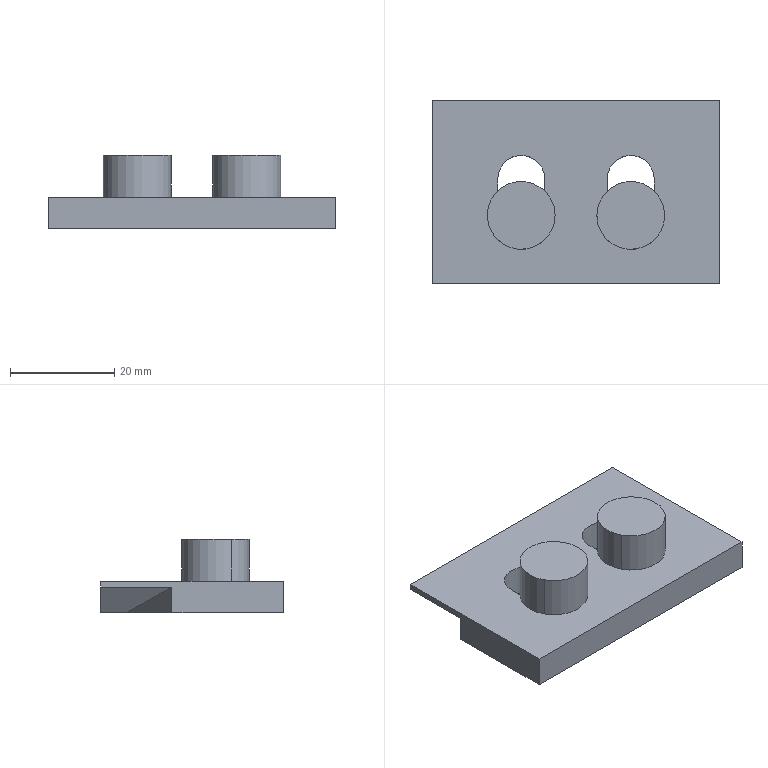Part | CATIA | 3 solids | 26 faces | box 55 x 35 x 14 mm | volume 11367 mm3 | plane 18 | cylinder 8 | commonest cylinder face diameters 9 x4 13 x4
STEP:
#1=CARTESIAN_POINT('',(-27.5,-30.,38.));
#2=VERTEX_POINT('',#1);
#3=CARTESIAN_POINT('',(-27.5,-30.,44.));
#4=VERTEX_POINT('',#3);
#5=CARTESIAN_POINT('',(-27.5,-30.,41.));
#6=DIRECTION('',(0.,0.,1.));
#7=VECTOR('',#6,1.);
#8=LINE('',#5,#7);
#9=EDGE_CURVE('',#2,#4,#8,.T.);
#10=ORIENTED_EDGE('',*,*,#9,.F.);
#11=CARTESIAN_POINT('',(27.5,-30.,38.));
#12=VERTEX_POINT('',#11);
#13=CARTESIAN_POINT('',(0.,-30.,38.));
#14=DIRECTION('',(1.,0.,0.));
#15=VECTOR('',#14,1.);
#16=LINE('',#13,#15);
#17=EDGE_CURVE('',#2,#12,#16,.T.);
#18=ORIENTED_EDGE('',*,*,#17,.T.);
#19=CARTESIAN_POINT('',(27.5,-30.,44.));
#20=VERTEX_POINT('',#19);
#21=CARTESIAN_POINT('',(27.5,-30.,41.));
#22=DIRECTION('',(0.,0.,1.));
#23=VECTOR('',#22,1.);
#24=LINE('',#21,#23);
#25=EDGE_CURVE('',#12,#20,#24,.T.);
#26=ORIENTED_EDGE('',*,*,#25,.T.);
#27=CARTESIAN_POINT('',(0.,-30.,44.));
#28=DIRECTION('',(1.,0.,0.));
#29=VECTOR('',#28,1.);
#30=LINE('',#27,#29);
#31=EDGE_CURVE('',#4,#20,#30,.T.);
#32=ORIENTED_EDGE('',*,*,#31,.F.);
#33=EDGE_LOOP('',(#10,#18,#26,#32));
#34=FACE_OUTER_BOUND('',#33,.T.);
#35=CARTESIAN_POINT('',(-27.5,-30.,38.));
#36=DIRECTION('',(0.,-1.,0.));
#37=DIRECTION('',(1.,0.,0.));
#38=AXIS2_PLACEMENT_3D('',#35,#36,#37);
#39=PLANE('',#38);
#40=ADVANCED_FACE('',(#34),#39,.T.);
#41=CARTESIAN_POINT('',(27.5,-8.66,42.874));
#42=VERTEX_POINT('',#41);
#43=CARTESIAN_POINT('',(27.5,-8.66,38.));
#44=VERTEX_POINT('',#43);
#45=CARTESIAN_POINT('',(27.5,-8.66,40.437));
#46=DIRECTION('',(0.,0.,-1.));
#47=VECTOR('',#46,1.);
#48=LINE('',#45,#47);
#49=EDGE_CURVE('',#42,#44,#48,.T.);
#50=ORIENTED_EDGE('',*,*,#49,.F.);
#51=CARTESIAN_POINT('',(27.5,5.,42.874));
#52=VERTEX_POINT('',#51);
#53=CARTESIAN_POINT('',(27.5,-1.83,42.874));
#54=DIRECTION('',(0.,1.,0.));
#55=VECTOR('',#54,1.);
#56=LINE('',#53,#55);
#57=EDGE_CURVE('',#42,#52,#56,.T.);
#58=ORIENTED_EDGE('',*,*,#57,.T.);
#59=CARTESIAN_POINT('',(27.5,5.,44.));
#60=VERTEX_POINT('',#59);
#61=CARTESIAN_POINT('',(27.5,5.,43.437));
#62=DIRECTION('',(0.,0.,1.));
#63=VECTOR('',#62,1.);
#64=LINE('',#61,#63);
#65=EDGE_CURVE('',#52,#60,#64,.T.);
#66=ORIENTED_EDGE('',*,*,#65,.T.);
#67=CARTESIAN_POINT('',(27.5,-12.5,44.));
#68=DIRECTION('',(0.,-1.,0.));
#69=VECTOR('',#68,1.);
#70=LINE('',#67,#69);
#71=EDGE_CURVE('',#20,#60,#70,.F.);
#72=ORIENTED_EDGE('',*,*,#71,.F.);
#73=ORIENTED_EDGE('',*,*,#25,.F.);
#74=CARTESIAN_POINT('',(27.5,-19.33,38.));
#75=DIRECTION('',(0.,-1.,0.));
#76=VECTOR('',#75,1.);
#77=LINE('',#74,#76);
#78=EDGE_CURVE('',#12,#44,#77,.F.);
#79=ORIENTED_EDGE('',*,*,#78,.T.);
#80=EDGE_LOOP('',(#50,#58,#66,#72,#73,#79));
#81=FACE_OUTER_BOUND('',#80,.T.);
#82=CARTESIAN_POINT('',(27.5,5.,38.));
#83=DIRECTION('',(-1.,0.,0.));
#84=DIRECTION('',(0.,-1.,0.));
#85=AXIS2_PLACEMENT_3D('',#82,#83,#84);
#86=PLANE('',#85);
#87=ADVANCED_FACE('',(#81),#86,.F.);
#88=CARTESIAN_POINT('',(-27.5,-8.66,42.874));
#89=VERTEX_POINT('',#88);
#90=CARTESIAN_POINT('',(-27.5,5.,42.874));
#91=VERTEX_POINT('',#90);
#92=CARTESIAN_POINT('',(-27.5,-1.83,42.874));
#93=DIRECTION('',(0.,1.,0.));
#94=VECTOR('',#93,1.);
#95=LINE('',#92,#94);
#96=EDGE_CURVE('',#89,#91,#95,.T.);
#97=ORIENTED_EDGE('',*,*,#96,.F.);
#98=CARTESIAN_POINT('',(-27.5,-8.66,38.));
#99=VERTEX_POINT('',#98);
#100=CARTESIAN_POINT('',(-27.5,-8.66,40.437));
#101=DIRECTION('',(0.,0.,-1.));
#102=VECTOR('',#101,1.);
#103=LINE('',#100,#102);
#104=EDGE_CURVE('',#89,#99,#103,.T.);
#105=ORIENTED_EDGE('',*,*,#104,.T.);
#106=CARTESIAN_POINT('',(-27.5,-19.33,38.));
#107=DIRECTION('',(0.,1.,0.));
#108=VECTOR('',#107,1.);
#109=LINE('',#106,#108);
#110=EDGE_CURVE('',#99,#2,#109,.F.);
#111=ORIENTED_EDGE('',*,*,#110,.T.);
#112=ORIENTED_EDGE('',*,*,#9,.T.);
#113=CARTESIAN_POINT('',(-27.5,5.,44.));
#114=VERTEX_POINT('',#113);
#115=CARTESIAN_POINT('',(-27.5,-12.5,44.));
#116=DIRECTION('',(0.,1.,0.));
#117=VECTOR('',#116,1.);
#118=LINE('',#115,#117);
#119=EDGE_CURVE('',#114,#4,#118,.F.);
#120=ORIENTED_EDGE('',*,*,#119,.F.);
#121=CARTESIAN_POINT('',(-27.5,5.,43.437));
#122=DIRECTION('',(0.,0.,1.));
#123=VECTOR('',#122,1.);
#124=LINE('',#121,#123);
#125=EDGE_CURVE('',#91,#114,#124,.T.);
#126=ORIENTED_EDGE('',*,*,#125,.F.);
#127=EDGE_LOOP('',(#97,#105,#111,#112,#120,#126));
#128=FACE_OUTER_BOUND('',#127,.T.);
#129=CARTESIAN_POINT('',(-27.5,-30.,38.));
#130=DIRECTION('',(1.,0.,0.));
#131=DIRECTION('',(0.,1.,0.));
#132=AXIS2_PLACEMENT_3D('',#129,#130,#131);
#133=PLANE('',#132);
#134=ADVANCED_FACE('',(#128),#133,.F.);
#135=CARTESIAN_POINT('',(12.5,5.,38.));
#136=VERTEX_POINT('',#135);
#137=CARTESIAN_POINT('',(-12.5,5.,38.));
#138=VERTEX_POINT('',#137);
#139=CARTESIAN_POINT('',(0.,5.,38.));
#140=DIRECTION('',(-1.,0.,0.));
#141=VECTOR('',#140,1.);
#142=LINE('',#139,#141);
#143=EDGE_CURVE('',#136,#138,#142,.T.);
#144=ORIENTED_EDGE('',*,*,#143,.T.);
#145=CARTESIAN_POINT('',(-20.,5.,40.437));
#146=DIRECTION('',(-0.9511,0.,0.309));
#147=VECTOR('',#146,1.);
#148=LINE('',#145,#147);
#149=EDGE_CURVE('',#138,#91,#148,.T.);
#150=ORIENTED_EDGE('',*,*,#149,.T.);
#151=ORIENTED_EDGE('',*,*,#125,.T.);
#152=CARTESIAN_POINT('',(0.,5.,44.));
#153=DIRECTION('',(-1.,0.,0.));
#154=VECTOR('',#153,1.);
#155=LINE('',#152,#154);
#156=EDGE_CURVE('',#60,#114,#155,.T.);
#157=ORIENTED_EDGE('',*,*,#156,.F.);
#158=ORIENTED_EDGE('',*,*,#65,.F.);
#159=CARTESIAN_POINT('',(20.,5.,40.437));
#160=DIRECTION('',(0.9511,0.,0.309));
#161=VECTOR('',#160,1.);
#162=LINE('',#159,#161);
#163=EDGE_CURVE('',#136,#52,#162,.T.);
#164=ORIENTED_EDGE('',*,*,#163,.F.);
#165=EDGE_LOOP('',(#144,#150,#151,#157,#158,#164));
#166=FACE_OUTER_BOUND('',#165,.T.);
#167=CARTESIAN_POINT('',(27.5,5.,38.));
#168=DIRECTION('',(0.,1.,0.));
#169=DIRECTION('',(-1.,0.,0.));
#170=AXIS2_PLACEMENT_3D('',#167,#168,#169);
#171=PLANE('',#170);
#172=ADVANCED_FACE('',(#166),#171,.T.);
#173=CARTESIAN_POINT('',(12.5,0.,38.));
#174=VERTEX_POINT('',#173);
#175=CARTESIAN_POINT('',(27.5,-8.66,42.874));
#176=CARTESIAN_POINT('',(12.5,0.,38.));
#177=B_SPLINE_CURVE_WITH_KNOTS('',1,(#175,#176),.UNSPECIFIED.,.F.,.U.,(2,2),(-2.999,14.994),.UNSPECIFIED.);
#178=EDGE_CURVE('',#174,#42,#177,.F.);
#179=ORIENTED_EDGE('',*,*,#178,.T.);
#180=ORIENTED_EDGE('',*,*,#49,.T.);
#181=CARTESIAN_POINT('',(25.,-7.217,38.));
#182=DIRECTION('',(0.866,-0.5,0.));
#183=VECTOR('',#182,1.);
#184=LINE('',#181,#183);
#185=EDGE_CURVE('',#174,#44,#184,.T.);
#186=ORIENTED_EDGE('',*,*,#185,.F.);
#187=EDGE_LOOP('',(#179,#180,#186));
#188=FACE_OUTER_BOUND('',#187,.T.);
#189=CARTESIAN_POINT('',(12.5,0.,38.));
#190=DIRECTION('',(0.5,0.866,0.));
#191=DIRECTION('',(0.,0.,1.));
#192=AXIS2_PLACEMENT_3D('',#189,#190,#191);
#193=PLANE('',#192);
#194=ADVANCED_FACE('',(#188),#193,.T.);
#195=ORIENTED_EDGE('',*,*,#163,.T.);
#196=ORIENTED_EDGE('',*,*,#57,.F.);
#197=ORIENTED_EDGE('',*,*,#178,.F.);
#198=CARTESIAN_POINT('',(12.5,5.,38.));
#199=DIRECTION('',(0.,-1.,0.));
#200=VECTOR('',#199,1.);
#201=LINE('',#198,#200);
#202=EDGE_CURVE('',#174,#136,#201,.F.);
#203=ORIENTED_EDGE('',*,*,#202,.T.);
#204=EDGE_LOOP('',(#195,#196,#197,#203));
#205=FACE_OUTER_BOUND('',#204,.T.);
#206=CARTESIAN_POINT('',(12.5,10.,38.));
#207=DIRECTION('',(-0.309,0.,0.9511));
#208=DIRECTION('',(0.,-1.,0.));
#209=AXIS2_PLACEMENT_3D('',#206,#207,#208);
#210=PLANE('',#209);
#211=ADVANCED_FACE('',(#205),#210,.F.);
#212=CARTESIAN_POINT('',(-12.5,0.,38.));
#213=VERTEX_POINT('',#212);
#214=CARTESIAN_POINT('',(-25.,-7.217,38.));
#215=DIRECTION('',(-0.866,-0.5,0.));
#216=VECTOR('',#215,1.);
#217=LINE('',#214,#216);
#218=EDGE_CURVE('',#213,#99,#217,.T.);
#219=ORIENTED_EDGE('',*,*,#218,.T.);
#220=ORIENTED_EDGE('',*,*,#104,.F.);
#221=CARTESIAN_POINT('',(-27.5,-8.66,42.874));
#222=CARTESIAN_POINT('',(-12.5,0.,38.));
#223=B_SPLINE_CURVE_WITH_KNOTS('',1,(#221,#222),.UNSPECIFIED.,.F.,.U.,(2,2),(-2.999,14.994),.UNSPECIFIED.);
#224=EDGE_CURVE('',#213,#89,#223,.F.);
#225=ORIENTED_EDGE('',*,*,#224,.F.);
#226=EDGE_LOOP('',(#219,#220,#225));
#227=FACE_OUTER_BOUND('',#226,.T.);
#228=CARTESIAN_POINT('',(-12.5,0.,38.));
#229=DIRECTION('',(0.5,-0.866,0.));
#230=DIRECTION('',(0.,0.,1.));
#231=AXIS2_PLACEMENT_3D('',#228,#229,#230);
#232=PLANE('',#231);
#233=ADVANCED_FACE('',(#227),#232,.F.);
#234=CARTESIAN_POINT('',(-12.5,5.,38.));
#235=DIRECTION('',(0.,-1.,0.));
#236=VECTOR('',#235,1.);
#237=LINE('',#234,#236);
#238=EDGE_CURVE('',#213,#138,#237,.F.);
#239=ORIENTED_EDGE('',*,*,#238,.F.);
#240=ORIENTED_EDGE('',*,*,#224,.T.);
#241=ORIENTED_EDGE('',*,*,#96,.T.);
#242=ORIENTED_EDGE('',*,*,#149,.F.);
#243=EDGE_LOOP('',(#239,#240,#241,#242));
#244=FACE_OUTER_BOUND('',#243,.T.);
#245=CARTESIAN_POINT('',(-12.5,10.,38.));
#246=DIRECTION('',(-0.309,0.,-0.9511));
#247=DIRECTION('',(0.,-1.,0.));
#248=AXIS2_PLACEMENT_3D('',#245,#246,#247);
#249=PLANE('',#248);
#250=ADVANCED_FACE('',(#244),#249,.T.);
#251=ORIENTED_EDGE('',*,*,#143,.F.);
#252=ORIENTED_EDGE('',*,*,#202,.F.);
#253=ORIENTED_EDGE('',*,*,#185,.T.);
#254=ORIENTED_EDGE('',*,*,#78,.F.);
#255=ORIENTED_EDGE('',*,*,#17,.F.);
#256=ORIENTED_EDGE('',*,*,#110,.F.);
#257=ORIENTED_EDGE('',*,*,#218,.F.);
#258=ORIENTED_EDGE('',*,*,#238,.T.);
#259=EDGE_LOOP('',(#251,#252,#253,#254,#255,#256,#257,#258));
#260=FACE_OUTER_BOUND('',#259,.T.);
#261=CARTESIAN_POINT('',(-6.,-10.,38.));
#262=VERTEX_POINT('',#261);
#263=CARTESIAN_POINT('',(-6.,-17.,38.));
#264=VERTEX_POINT('',#263);
#265=CARTESIAN_POINT('',(-6.,-13.5,38.));
#266=DIRECTION('',(0.,-1.,0.));
#267=VECTOR('',#266,1.);
#268=LINE('',#265,#267);
#269=EDGE_CURVE('',#262,#264,#268,.T.);
#270=ORIENTED_EDGE('',*,*,#269,.F.);
#271=CARTESIAN_POINT('',(-15.,-10.,38.));
#272=VERTEX_POINT('',#271);
#273=CARTESIAN_POINT('',(-10.5,-10.,38.));
#274=DIRECTION('',(0.,0.,1.));
#275=AXIS2_PLACEMENT_3D('',#273,#274,$);
#276=CIRCLE('',#275,4.5);
#277=EDGE_CURVE('',#262,#272,#276,.T.);
#278=ORIENTED_EDGE('',*,*,#277,.T.);
#279=CARTESIAN_POINT('',(-15.,-17.,38.));
#280=VERTEX_POINT('',#279);
#281=CARTESIAN_POINT('',(-15.,-13.5,38.));
#282=DIRECTION('',(0.,-1.,0.));
#283=VECTOR('',#282,1.);
#284=LINE('',#281,#283);
#285=EDGE_CURVE('',#272,#280,#284,.T.);
#286=ORIENTED_EDGE('',*,*,#285,.T.);
#287=CARTESIAN_POINT('',(-10.5,-17.,38.));
#288=DIRECTION('',(0.,0.,1.));
#289=AXIS2_PLACEMENT_3D('',#287,#288,$);
#290=CIRCLE('',#289,4.5);
#291=EDGE_CURVE('',#280,#264,#290,.T.);
#292=ORIENTED_EDGE('',*,*,#291,.T.);
#293=EDGE_LOOP('',(#270,#278,#286,#292));
#294=FACE_BOUND('',#293,.T.);
#295=CARTESIAN_POINT('',(15.,-10.,38.));
#296=VERTEX_POINT('',#295);
#297=CARTESIAN_POINT('',(6.,-10.,38.));
#298=VERTEX_POINT('',#297);
#299=CARTESIAN_POINT('',(10.5,-10.,38.));
#300=DIRECTION('',(0.,0.,1.));
#301=AXIS2_PLACEMENT_3D('',#299,#300,$);
#302=CIRCLE('',#301,4.5);
#303=EDGE_CURVE('',#296,#298,#302,.T.);
#304=ORIENTED_EDGE('',*,*,#303,.T.);
#305=CARTESIAN_POINT('',(6.,-17.,38.));
#306=VERTEX_POINT('',#305);
#307=CARTESIAN_POINT('',(6.,-13.5,38.));
#308=DIRECTION('',(0.,-1.,0.));
#309=VECTOR('',#308,1.);
#310=LINE('',#307,#309);
#311=EDGE_CURVE('',#298,#306,#310,.T.);
#312=ORIENTED_EDGE('',*,*,#311,.T.);
#313=CARTESIAN_POINT('',(15.,-17.,38.));
#314=VERTEX_POINT('',#313);
#315=CARTESIAN_POINT('',(10.5,-17.,38.));
#316=DIRECTION('',(0.,0.,1.));
#317=AXIS2_PLACEMENT_3D('',#315,#316,$);
#318=CIRCLE('',#317,4.5);
#319=EDGE_CURVE('',#306,#314,#318,.T.);
#320=ORIENTED_EDGE('',*,*,#319,.T.);
#321=CARTESIAN_POINT('',(15.,-13.5,38.));
#322=DIRECTION('',(0.,-1.,0.));
#323=VECTOR('',#322,1.);
#324=LINE('',#321,#323);
#325=EDGE_CURVE('',#296,#314,#324,.T.);
#326=ORIENTED_EDGE('',*,*,#325,.F.);
#327=EDGE_LOOP('',(#304,#312,#320,#326));
#328=FACE_BOUND('',#327,.T.);
#329=CARTESIAN_POINT('',(0.,0.,38.));
#330=DIRECTION('',(0.,0.,1.));
#331=DIRECTION('',(1.,0.,0.));
#332=AXIS2_PLACEMENT_3D('',#329,#330,#331);
#333=PLANE('',#332);
#334=ADVANCED_FACE('',(#260,#294,#328),#333,.F.);
#335=ORIENTED_EDGE('',*,*,#156,.T.);
#336=ORIENTED_EDGE('',*,*,#119,.T.);
#337=ORIENTED_EDGE('',*,*,#31,.T.);
#338=ORIENTED_EDGE('',*,*,#71,.T.);
#339=EDGE_LOOP('',(#335,#336,#337,#338));
#340=FACE_OUTER_BOUND('',#339,.T.);
#341=CARTESIAN_POINT('',(-6.,-17.,44.));
#342=VERTEX_POINT('',#341);
#343=CARTESIAN_POINT('',(-6.,-10.,44.));
#344=VERTEX_POINT('',#343);
#345=CARTESIAN_POINT('',(-6.,-13.5,44.));
#346=DIRECTION('',(0.,-1.,0.));
#347=VECTOR('',#346,1.);
#348=LINE('',#345,#347);
#349=EDGE_CURVE('',#342,#344,#348,.F.);
#350=ORIENTED_EDGE('',*,*,#349,.F.);
#351=CARTESIAN_POINT('',(-15.,-17.,44.));
#352=VERTEX_POINT('',#351);
#353=CARTESIAN_POINT('',(-10.5,-17.,44.));
#354=DIRECTION('',(0.,0.,1.));
#355=AXIS2_PLACEMENT_3D('',#353,#354,$);
#356=CIRCLE('',#355,4.5);
#357=EDGE_CURVE('',#352,#342,#356,.T.);
#358=ORIENTED_EDGE('',*,*,#357,.F.);
#359=CARTESIAN_POINT('',(-15.,-10.,44.));
#360=VERTEX_POINT('',#359);
#361=CARTESIAN_POINT('',(-15.,-13.5,44.));
#362=DIRECTION('',(0.,-1.,0.));
#363=VECTOR('',#362,1.);
#364=LINE('',#361,#363);
#365=EDGE_CURVE('',#360,#352,#364,.T.);
#366=ORIENTED_EDGE('',*,*,#365,.F.);
#367=CARTESIAN_POINT('',(-10.5,-10.,44.));
#368=DIRECTION('',(0.,0.,1.));
#369=AXIS2_PLACEMENT_3D('',#367,#368,$);
#370=CIRCLE('',#369,4.5);
#371=EDGE_CURVE('',#344,#360,#370,.T.);
#372=ORIENTED_EDGE('',*,*,#371,.F.);
#373=EDGE_LOOP('',(#350,#358,#366,#372));
#374=FACE_BOUND('',#373,.T.);
#375=CARTESIAN_POINT('',(15.,-10.,44.));
#376=VERTEX_POINT('',#375);
#377=CARTESIAN_POINT('',(6.,-10.,44.));
#378=VERTEX_POINT('',#377);
#379=CARTESIAN_POINT('',(10.5,-10.,44.));
#380=DIRECTION('',(0.,0.,1.));
#381=AXIS2_PLACEMENT_3D('',#379,#380,$);
#382=CIRCLE('',#381,4.5);
#383=EDGE_CURVE('',#376,#378,#382,.T.);
#384=ORIENTED_EDGE('',*,*,#383,.F.);
#385=CARTESIAN_POINT('',(15.,-17.,44.));
#386=VERTEX_POINT('',#385);
#387=CARTESIAN_POINT('',(15.,-13.5,44.));
#388=DIRECTION('',(0.,-1.,0.));
#389=VECTOR('',#388,1.);
#390=LINE('',#387,#389);
#391=EDGE_CURVE('',#386,#376,#390,.F.);
#392=ORIENTED_EDGE('',*,*,#391,.F.);
#393=CARTESIAN_POINT('',(6.,-17.,44.));
#394=VERTEX_POINT('',#393);
#395=CARTESIAN_POINT('',(10.5,-17.,44.));
#396=DIRECTION('',(0.,0.,1.));
#397=AXIS2_PLACEMENT_3D('',#395,#396,$);
#398=CIRCLE('',#397,4.5);
#399=EDGE_CURVE('',#394,#386,#398,.T.);
#400=ORIENTED_EDGE('',*,*,#399,.F.);
#401=CARTESIAN_POINT('',(6.,-13.5,44.));
#402=DIRECTION('',(0.,-1.,0.));
#403=VECTOR('',#402,1.);
#404=LINE('',#401,#403);
#405=EDGE_CURVE('',#378,#394,#404,.T.);
#406=ORIENTED_EDGE('',*,*,#405,.F.);
#407=EDGE_LOOP('',(#384,#392,#400,#406));
#408=FACE_BOUND('',#407,.T.);
#409=CARTESIAN_POINT('',(0.,0.,44.));
#410=DIRECTION('',(0.,0.,1.));
#411=DIRECTION('',(1.,0.,0.));
#412=AXIS2_PLACEMENT_3D('',#409,#410,#411);
#413=PLANE('',#412);
#414=ADVANCED_FACE('',(#340,#374,#408),#413,.T.);
#415=ORIENTED_EDGE('',*,*,#303,.F.);
#416=CARTESIAN_POINT('',(15.,-10.,34.));
#417=DIRECTION('',(0.,0.,1.));
#418=VECTOR('',#417,1.);
#419=LINE('',#416,#418);
#420=EDGE_CURVE('',#376,#296,#419,.F.);
#421=ORIENTED_EDGE('',*,*,#420,.F.);
#422=ORIENTED_EDGE('',*,*,#383,.T.);
#423=CARTESIAN_POINT('',(6.,-10.,34.));
#424=DIRECTION('',(0.,0.,1.));
#425=VECTOR('',#424,1.);
#426=LINE('',#423,#425);
#427=EDGE_CURVE('',#378,#298,#426,.F.);
#428=ORIENTED_EDGE('',*,*,#427,.T.);
#429=EDGE_LOOP('',(#415,#421,#422,#428));
#430=FACE_OUTER_BOUND('',#429,.T.);
#431=CARTESIAN_POINT('',(10.5,-10.,34.));
#432=DIRECTION('',(0.,0.,1.));
#433=DIRECTION('',(1.,0.,0.));
#434=AXIS2_PLACEMENT_3D('',#431,#432,#433);
#435=CYLINDRICAL_SURFACE('',#434,4.5);
#436=ADVANCED_FACE('',(#430),#435,.F.);
#437=ORIENTED_EDGE('',*,*,#427,.F.);
#438=ORIENTED_EDGE('',*,*,#405,.T.);
#439=CARTESIAN_POINT('',(6.,-17.,41.));
#440=DIRECTION('',(0.,0.,-1.));
#441=VECTOR('',#440,1.);
#442=LINE('',#439,#441);
#443=EDGE_CURVE('',#394,#306,#442,.T.);
#444=ORIENTED_EDGE('',*,*,#443,.T.);
#445=ORIENTED_EDGE('',*,*,#311,.F.);
#446=EDGE_LOOP('',(#437,#438,#444,#445));
#447=FACE_OUTER_BOUND('',#446,.T.);
#448=CARTESIAN_POINT('',(6.,-10.,44.));
#449=DIRECTION('',(1.,0.,0.));
#450=DIRECTION('',(0.,-1.,0.));
#451=AXIS2_PLACEMENT_3D('',#448,#449,#450);
#452=PLANE('',#451);
#453=ADVANCED_FACE('',(#447),#452,.T.);
#454=ORIENTED_EDGE('',*,*,#325,.T.);
#455=CARTESIAN_POINT('',(15.,-17.,41.));
#456=DIRECTION('',(0.,0.,-1.));
#457=VECTOR('',#456,1.);
#458=LINE('',#455,#457);
#459=EDGE_CURVE('',#386,#314,#458,.T.);
#460=ORIENTED_EDGE('',*,*,#459,.F.);
#461=ORIENTED_EDGE('',*,*,#391,.T.);
#462=ORIENTED_EDGE('',*,*,#420,.T.);
#463=EDGE_LOOP('',(#454,#460,#461,#462));
#464=FACE_OUTER_BOUND('',#463,.T.);
#465=CARTESIAN_POINT('',(15.,-10.,44.));
#466=DIRECTION('',(1.,0.,0.));
#467=DIRECTION('',(0.,-1.,0.));
#468=AXIS2_PLACEMENT_3D('',#465,#466,#467);
#469=PLANE('',#468);
#470=ADVANCED_FACE('',(#464),#469,.F.);
#471=ORIENTED_EDGE('',*,*,#319,.F.);
#472=ORIENTED_EDGE('',*,*,#443,.F.);
#473=ORIENTED_EDGE('',*,*,#399,.T.);
#474=ORIENTED_EDGE('',*,*,#459,.T.);
#475=EDGE_LOOP('',(#471,#472,#473,#474));
#476=FACE_OUTER_BOUND('',#475,.T.);
#477=CARTESIAN_POINT('',(10.5,-17.,34.));
#478=DIRECTION('',(0.,0.,1.));
#479=DIRECTION('',(-1.,0.,0.));
#480=AXIS2_PLACEMENT_3D('',#477,#478,#479);
#481=CYLINDRICAL_SURFACE('',#480,4.5);
#482=ADVANCED_FACE('',(#476),#481,.F.);
#483=ORIENTED_EDGE('',*,*,#269,.T.);
#484=CARTESIAN_POINT('',(-6.,-17.,41.));
#485=DIRECTION('',(0.,0.,-1.));
#486=VECTOR('',#485,1.);
#487=LINE('',#484,#486);
#488=EDGE_CURVE('',#342,#264,#487,.T.);
#489=ORIENTED_EDGE('',*,*,#488,.F.);
#490=ORIENTED_EDGE('',*,*,#349,.T.);
#491=CARTESIAN_POINT('',(-6.,-10.,41.));
#492=DIRECTION('',(0.,0.,-1.));
#493=VECTOR('',#492,1.);
#494=LINE('',#491,#493);
#495=EDGE_CURVE('',#344,#262,#494,.T.);
#496=ORIENTED_EDGE('',*,*,#495,.T.);
#497=EDGE_LOOP('',(#483,#489,#490,#496));
#498=FACE_OUTER_BOUND('',#497,.T.);
#499=CARTESIAN_POINT('',(-6.,-10.,44.));
#500=DIRECTION('',(1.,0.,0.));
#501=DIRECTION('',(0.,-1.,0.));
#502=AXIS2_PLACEMENT_3D('',#499,#500,#501);
#503=PLANE('',#502);
#504=ADVANCED_FACE('',(#498),#503,.F.);
#505=ORIENTED_EDGE('',*,*,#277,.F.);
#506=ORIENTED_EDGE('',*,*,#495,.F.);
#507=ORIENTED_EDGE('',*,*,#371,.T.);
#508=CARTESIAN_POINT('',(-15.,-10.,34.));
#509=DIRECTION('',(0.,0.,1.));
#510=VECTOR('',#509,1.);
#511=LINE('',#508,#510);
#512=EDGE_CURVE('',#360,#272,#511,.F.);
#513=ORIENTED_EDGE('',*,*,#512,.T.);
#514=EDGE_LOOP('',(#505,#506,#507,#513));
#515=FACE_OUTER_BOUND('',#514,.T.);
#516=CARTESIAN_POINT('',(-10.5,-10.,34.));
#517=DIRECTION('',(0.,0.,1.));
#518=DIRECTION('',(1.,0.,0.));
#519=AXIS2_PLACEMENT_3D('',#516,#517,#518);
#520=CYLINDRICAL_SURFACE('',#519,4.5);
#521=ADVANCED_FACE('',(#515),#520,.F.);
#522=ORIENTED_EDGE('',*,*,#291,.F.);
#523=CARTESIAN_POINT('',(-15.,-17.,34.));
#524=DIRECTION('',(0.,0.,1.));
#525=VECTOR('',#524,1.);
#526=LINE('',#523,#525);
#527=EDGE_CURVE('',#352,#280,#526,.F.);
#528=ORIENTED_EDGE('',*,*,#527,.F.);
#529=ORIENTED_EDGE('',*,*,#357,.T.);
#530=ORIENTED_EDGE('',*,*,#488,.T.);
#531=EDGE_LOOP('',(#522,#528,#529,#530));
#532=FACE_OUTER_BOUND('',#531,.T.);
#533=CARTESIAN_POINT('',(-10.5,-17.,34.));
#534=DIRECTION('',(0.,0.,1.));
#535=DIRECTION('',(-1.,0.,0.));
#536=AXIS2_PLACEMENT_3D('',#533,#534,#535);
#537=CYLINDRICAL_SURFACE('',#536,4.5);
#538=ADVANCED_FACE('',(#532),#537,.F.);
#539=ORIENTED_EDGE('',*,*,#512,.F.);
#540=ORIENTED_EDGE('',*,*,#365,.T.);
#541=ORIENTED_EDGE('',*,*,#527,.T.);
#542=ORIENTED_EDGE('',*,*,#285,.F.);
#543=EDGE_LOOP('',(#539,#540,#541,#542));
#544=FACE_OUTER_BOUND('',#543,.T.);
#545=CARTESIAN_POINT('',(-15.,-10.,44.));
#546=DIRECTION('',(1.,0.,0.));
#547=DIRECTION('',(0.,-1.,0.));
#548=AXIS2_PLACEMENT_3D('',#545,#546,#547);
#549=PLANE('',#548);
#550=ADVANCED_FACE('',(#544),#549,.T.);
#551=CLOSED_SHELL('',(#40,#87,#134,#172,#194,#211,#233,#250,#334,#414,#436,#453,#470,#482,#504,#521,#538,#550));
#552=MANIFOLD_SOLID_BREP('',#551);
#553=CARTESIAN_POINT('',(-4.796,-13.884,52.));
#554=VERTEX_POINT('',#553);
#555=CARTESIAN_POINT('',(-16.204,-20.116,52.));
#556=VERTEX_POINT('',#555);
#557=CARTESIAN_POINT('',(-10.5,-17.,52.));
#558=DIRECTION('',(0.,0.,1.));
#559=AXIS2_PLACEMENT_3D('',#557,#558,$);
#560=CIRCLE('',#559,6.5);
#561=EDGE_CURVE('',#554,#556,#560,.T.);
#562=ORIENTED_EDGE('',*,*,#561,.T.);
#563=CARTESIAN_POINT('',(-10.5,-17.,52.));
#564=DIRECTION('',(0.,0.,1.));
#565=AXIS2_PLACEMENT_3D('',#563,#564,$);
#566=CIRCLE('',#565,6.5);
#567=EDGE_CURVE('',#556,#554,#566,.T.);
#568=ORIENTED_EDGE('',*,*,#567,.T.);
#569=EDGE_LOOP('',(#562,#568));
#570=FACE_OUTER_BOUND('',#569,.T.);
#571=CARTESIAN_POINT('',(-10.5,-17.,52.));
#572=DIRECTION('',(0.,0.,1.));
#573=DIRECTION('',(1.,0.,0.));
#574=AXIS2_PLACEMENT_3D('',#571,#572,#573);
#575=PLANE('',#574);
#576=ADVANCED_FACE('',(#570),#575,.T.);
#577=CARTESIAN_POINT('',(-16.204,-20.116,44.));
#578=VERTEX_POINT('',#577);
#579=CARTESIAN_POINT('',(-16.204,-20.116,47.8));
#580=DIRECTION('',(0.,0.,1.));
#581=VECTOR('',#580,1.);
#582=LINE('',#579,#581);
#583=EDGE_CURVE('',#556,#578,#582,.F.);
#584=ORIENTED_EDGE('',*,*,#583,.F.);
#585=ORIENTED_EDGE('',*,*,#561,.F.);
#586=CARTESIAN_POINT('',(-4.796,-13.884,44.));
#587=VERTEX_POINT('',#586);
#588=CARTESIAN_POINT('',(-4.796,-13.884,47.8));
#589=DIRECTION('',(0.,0.,1.));
#590=VECTOR('',#589,1.);
#591=LINE('',#588,#590);
#592=EDGE_CURVE('',#554,#587,#591,.F.);
#593=ORIENTED_EDGE('',*,*,#592,.T.);
#594=CARTESIAN_POINT('',(-10.5,-17.,44.));
#595=DIRECTION('',(0.,0.,1.));
#596=AXIS2_PLACEMENT_3D('',#594,#595,$);
#597=CIRCLE('',#596,6.5);
#598=EDGE_CURVE('',#587,#578,#597,.T.);
#599=ORIENTED_EDGE('',*,*,#598,.T.);
#600=EDGE_LOOP('',(#584,#585,#593,#599));
#601=FACE_OUTER_BOUND('',#600,.T.);
#602=CARTESIAN_POINT('',(-10.5,-17.,44.1));
#603=DIRECTION('',(0.,0.,1.));
#604=DIRECTION('',(0.8776,0.4794,0.));
#605=AXIS2_PLACEMENT_3D('',#602,#603,#604);
#606=CYLINDRICAL_SURFACE('',#605,6.5);
#607=ADVANCED_FACE('',(#601),#606,.T.);
#608=ORIENTED_EDGE('',*,*,#592,.F.);
#609=ORIENTED_EDGE('',*,*,#567,.F.);
#610=ORIENTED_EDGE('',*,*,#583,.T.);
#611=CARTESIAN_POINT('',(-10.5,-17.,44.));
#612=DIRECTION('',(0.,0.,1.));
#613=AXIS2_PLACEMENT_3D('',#611,#612,$);
#614=CIRCLE('',#613,6.5);
#615=EDGE_CURVE('',#578,#587,#614,.T.);
#616=ORIENTED_EDGE('',*,*,#615,.T.);
#617=EDGE_LOOP('',(#608,#609,#610,#616));
#618=FACE_OUTER_BOUND('',#617,.T.);
#619=ADVANCED_FACE('',(#618),#606,.T.);
#620=ORIENTED_EDGE('',*,*,#598,.F.);
#621=ORIENTED_EDGE('',*,*,#615,.F.);
#622=EDGE_LOOP('',(#620,#621));
#623=FACE_OUTER_BOUND('',#622,.T.);
#624=ADVANCED_FACE('',(#623),#413,.F.);
#625=CLOSED_SHELL('',(#576,#607,#619,#624));
#626=MANIFOLD_SOLID_BREP('',#625);
#627=CARTESIAN_POINT('',(16.204,-13.884,52.));
#628=VERTEX_POINT('',#627);
#629=CARTESIAN_POINT('',(4.796,-20.116,52.));
#630=VERTEX_POINT('',#629);
#631=CARTESIAN_POINT('',(10.5,-17.,52.));
#632=DIRECTION('',(0.,0.,1.));
#633=AXIS2_PLACEMENT_3D('',#631,#632,$);
#634=CIRCLE('',#633,6.5);
#635=EDGE_CURVE('',#628,#630,#634,.T.);
#636=ORIENTED_EDGE('',*,*,#635,.T.);
#637=CARTESIAN_POINT('',(10.5,-17.,52.));
#638=DIRECTION('',(0.,0.,1.));
#639=AXIS2_PLACEMENT_3D('',#637,#638,$);
#640=CIRCLE('',#639,6.5);
#641=EDGE_CURVE('',#630,#628,#640,.T.);
#642=ORIENTED_EDGE('',*,*,#641,.T.);
#643=EDGE_LOOP('',(#636,#642));
#644=FACE_OUTER_BOUND('',#643,.T.);
#645=ADVANCED_FACE('',(#644),#575,.T.);
#646=CARTESIAN_POINT('',(4.796,-20.116,44.));
#647=VERTEX_POINT('',#646);
#648=CARTESIAN_POINT('',(4.796,-20.116,47.8));
#649=DIRECTION('',(0.,0.,1.));
#650=VECTOR('',#649,1.);
#651=LINE('',#648,#650);
#652=EDGE_CURVE('',#630,#647,#651,.F.);
#653=ORIENTED_EDGE('',*,*,#652,.F.);
#654=ORIENTED_EDGE('',*,*,#635,.F.);
#655=CARTESIAN_POINT('',(16.204,-13.884,44.));
#656=VERTEX_POINT('',#655);
#657=CARTESIAN_POINT('',(16.204,-13.884,47.8));
#658=DIRECTION('',(0.,0.,1.));
#659=VECTOR('',#658,1.);
#660=LINE('',#657,#659);
#661=EDGE_CURVE('',#628,#656,#660,.F.);
#662=ORIENTED_EDGE('',*,*,#661,.T.);
#663=CARTESIAN_POINT('',(10.5,-17.,44.));
#664=DIRECTION('',(0.,0.,1.));
#665=AXIS2_PLACEMENT_3D('',#663,#664,$);
#666=CIRCLE('',#665,6.5);
#667=EDGE_CURVE('',#656,#647,#666,.T.);
#668=ORIENTED_EDGE('',*,*,#667,.T.);
#669=EDGE_LOOP('',(#653,#654,#662,#668));
#670=FACE_OUTER_BOUND('',#669,.T.);
#671=CARTESIAN_POINT('',(10.5,-17.,44.1));
#672=DIRECTION('',(0.,0.,1.));
#673=DIRECTION('',(0.8776,0.4794,0.));
#674=AXIS2_PLACEMENT_3D('',#671,#672,#673);
#675=CYLINDRICAL_SURFACE('',#674,6.5);
#676=ADVANCED_FACE('',(#670),#675,.T.);
#677=ORIENTED_EDGE('',*,*,#661,.F.);
#678=ORIENTED_EDGE('',*,*,#641,.F.);
#679=ORIENTED_EDGE('',*,*,#652,.T.);
#680=CARTESIAN_POINT('',(10.5,-17.,44.));
#681=DIRECTION('',(0.,0.,1.));
#682=AXIS2_PLACEMENT_3D('',#680,#681,$);
#683=CIRCLE('',#682,6.5);
#684=EDGE_CURVE('',#647,#656,#683,.T.);
#685=ORIENTED_EDGE('',*,*,#684,.T.);
#686=EDGE_LOOP('',(#677,#678,#679,#685));
#687=FACE_OUTER_BOUND('',#686,.T.);
#688=ADVANCED_FACE('',(#687),#675,.T.);
#689=ORIENTED_EDGE('',*,*,#667,.F.);
#690=ORIENTED_EDGE('',*,*,#684,.F.);
#691=EDGE_LOOP('',(#689,#690));
#692=FACE_OUTER_BOUND('',#691,.T.);
#693=ADVANCED_FACE('',(#692),#413,.F.);
#694=CLOSED_SHELL('',(#645,#676,#688,#693));
#695=MANIFOLD_SOLID_BREP('',#694);
#696=(LENGTH_UNIT()NAMED_UNIT(*)SI_UNIT(.MILLI.,.METRE.));
#697=UNCERTAINTY_MEASURE_WITH_UNIT(LENGTH_MEASURE(0.005),#696,'','');
#698=(NAMED_UNIT(*)PLANE_ANGLE_UNIT()SI_UNIT($,.RADIAN.));
#699=(NAMED_UNIT(*)SI_UNIT($,.STERADIAN.)SOLID_ANGLE_UNIT());
#700=(GEOMETRIC_REPRESENTATION_CONTEXT(3)GLOBAL_UNCERTAINTY_ASSIGNED_CONTEXT((#697))GLOBAL_UNIT_ASSIGNED_CONTEXT((#696,#698,#699))REPRESENTATION_CONTEXT('',''));
#701=ADVANCED_BREP_SHAPE_REPRESENTATION('',(#552,#626,#695),#700);